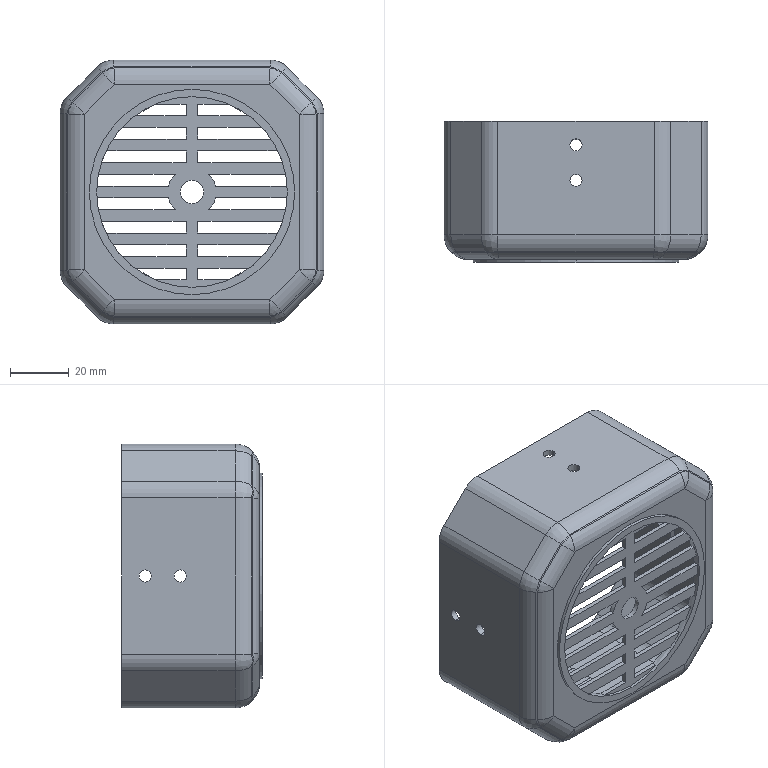Part | STEP file | 1 solid | 231 faces | box 90 x 48 x 90 mm | volume 30003 mm3 | plane 109 | cylinder 90 | spline 32 | commonest cylinder face diameters 13 x32 16 x32 4.1 x16 16.56 x4 8 x2 65 x2